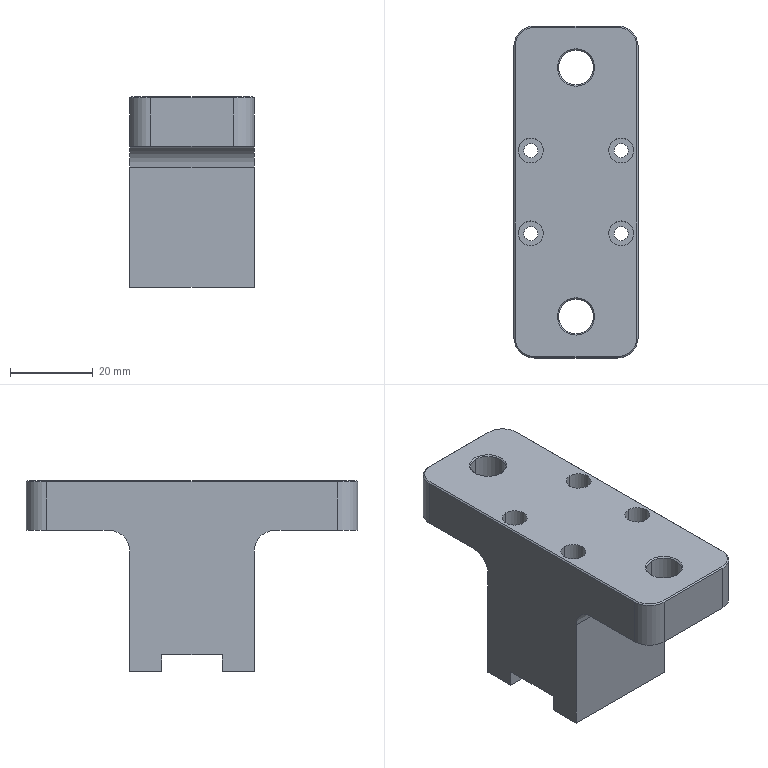NC program | NX | posted with a generic post | part box 30 x 80 x 46 mm
Whole program:
N10 G17 G21 G94 G90
(FLOOR_WALL_COPY_COPY , TOOL : D80)
N12 T19 M6
N14 G54
N16 G17 G0 G90 X-85. Y0. S6500 M3
N18 G43 Z30. H19
N20 Z6.
N22 G94 G1 Z3. F1500.
N24 X-80.
N26 X80.
N28 X85.
N30 Z6.
N32 G0 Z30.
N34 X-85.
N36 Z5.
N38 G1 Z2.
N40 X-80.
N42 X80.
N44 X85.
N46 Z5.
N48 G0 Z30.
N50 X-85.
N52 Z4.
N54 G1 Z1.
N56 X-80.
N58 X80.
N60 X85.
N62 Z4.
N64 G0 Z30.
N66 X-85.
N68 Z3.
N70 G1 Z0.
N72 X-80.
N74 X80.
N76 X85.
N78 Z3.
N80 G0 Z30.
N82 M5
(DRILLING_COPY_1_COPY_COPY_COPY , TOOL : 6.0ZT)
N84 T06 M6
N86 G54
N88 G17 G0 G90 X-10. Y10.9 S2000 M3
N90 G43 Z30. H6
N92 G94 G83 G98 Z-35.803 F100. Q2. R3.
N94 X10.
N96 X-10. Y-10.9
N98 X10.
N100 G80
N102 G0 X10. Y-10.9 Z30.
N104 M5
(PLANAR_MILL_COPY_COPY_COPY_COPY_COPY_COPY_1_COPY_1_COPY_1 , TOOL : D6A45)
N106 T01 M6
N108 G54
N110 G17 G0 G90 X33. Y-0.866 S9500 M3
N112 G43 Z30. H1
N114 Z0.5
N116 G94 G1 Z-1. F1250.
N118 G3 X33.5 Y0. R1.
N120 X30. Y3.5 R3.5
N122 X33.5 Y0. R-3.5
N124 X33. Y0.866 R1.
N126 G1 Z0.5
N128 G0 Z30.
N130 X9.134 Y-12.7
N132 Z0.5
N134 G1 Z-1.
N136 G3 X10. Y-13.2 R1.
N138 X12.3 Y-10.9 R2.3
N140 X10. Y-13.2 R-2.3
N142 X10.866 Y-12.7 R1.
N144 G1 Z0.5
N146 G0 Z30.
N148 X-10.866
N150 Z0.5
N152 G1 Z-1.
N154 G3 X-10. Y-13.2 R1.
N156 X-7.7 Y-10.9 R2.3
N158 X-10. Y-13.2 R-2.3
N160 X-9.134 Y-12.7 R1.
N162 G1 Z0.5
N164 G0 Z30.
N166 X0.866 Y-16.2
N168 Z0.5
N170 G1 Z-1.
N172 G3 X0. Y-15.7 R1.
N174 G1 X-35.
N176 G2 X-40.7 Y-10. R5.7
N178 G1 Y10.
N180 G2 X-35. Y15.7 R5.7
N182 G1 X35.
N184 G2 X40.7 Y10. R5.7
N186 G1 Y-10.
N188 G2 X35. Y-15.7 R5.7
N190 G1 X0.
N192 G3 X-0.866 Y-16.2 R1.
N194 G1 Z0.5
N196 G0 Z30.
N198 X10.866 Y12.7
N200 Z0.5
N202 G1 Z-1.
N204 G3 X10. Y13.2 R1.
N206 X7.7 Y10.9 R2.3
N208 X10. Y13.2 R-2.3
N210 X9.134 Y12.7 R1.
N212 G1 Z0.5
N214 G0 Z30.
N216 X-9.134
N218 Z0.5
N220 G1 Z-1.
N222 G3 X-10. Y13.2 R1.
N224 X-12.3 Y10.9 R2.3
N226 X-10. Y13.2 R-2.3
N228 X-10.866 Y12.7 R1.
N230 G1 Z0.5
N232 G0 Z30.
N234 X-33. Y0.866
N236 Z0.5
N238 G1 Z-1.
N240 G3 X-33.5 Y0. R1.
N242 X-30. Y-3.5 R3.5
N244 X-33.5 Y0. R-3.5
N246 X-33. Y-0.866 R1.
N248 G1 Z0.5
N250 G0 Z30.
N252 M5
N254 M2